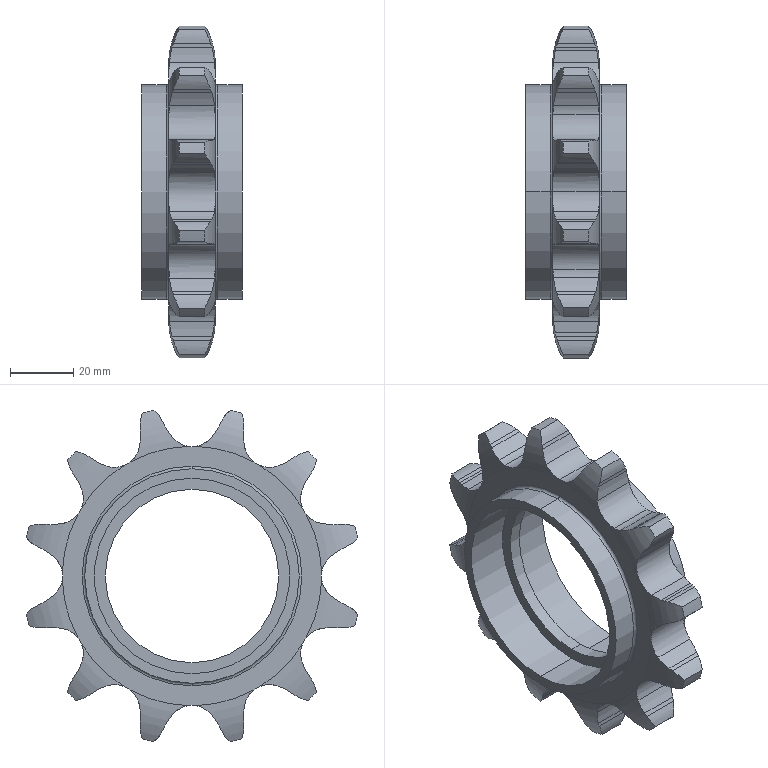Part | STEP file | Driven sprocket 16A-12_05B | 1 solid | 147 faces | box 32 x 105.245 x 105.245 mm | volume 65357 mm3 | cylinder 89 | plane 30 | torus 28 | commonest cylinder face diameters 23.691 x26 41.467 x26 16.059 x15 108 x12 62 x4 68 x4